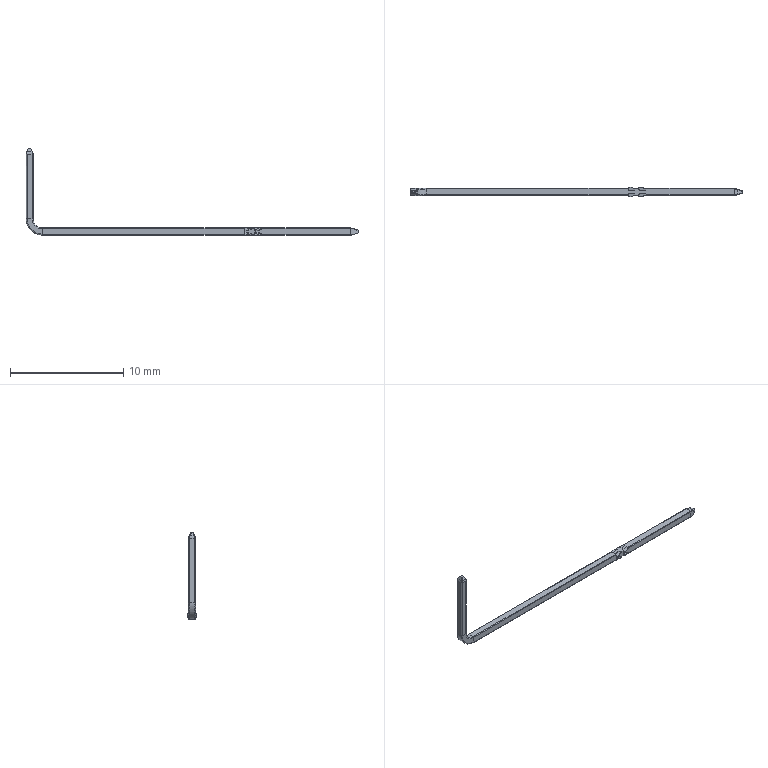Part | NX | features BREP 1 | 1 solid | 204 faces | box 29.315 x 0.8779 x 7.616 mm | volume 13.838 mm3 | cylinder 82 | plane 74 | torus 22 | sphere 20 | spline 6 | commonest cylinder face diameters 0.09 x28 0.1 x24 0.2 x12 2.01 x8 1 x4 2 x4